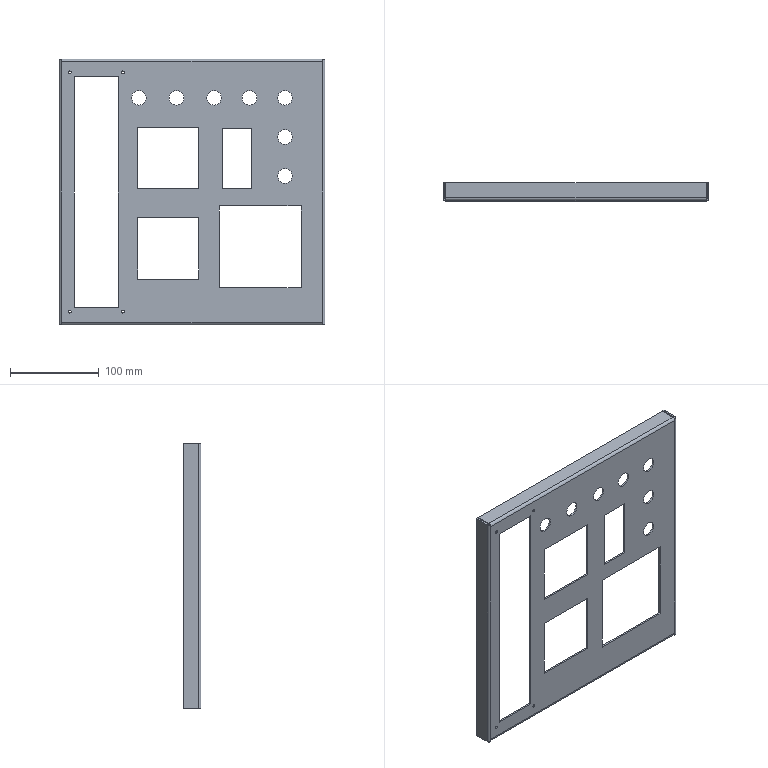Part | STEP file | Station two ctrl box cover | 1 solid | 82 faces | box 300 x 20 x 300 mm | volume 151242 mm3 | plane 48 | cylinder 34 | commonest cylinder face diameters 16.5 x14 3.3 x8 2 x4 6 x4 5 x2 9 x2